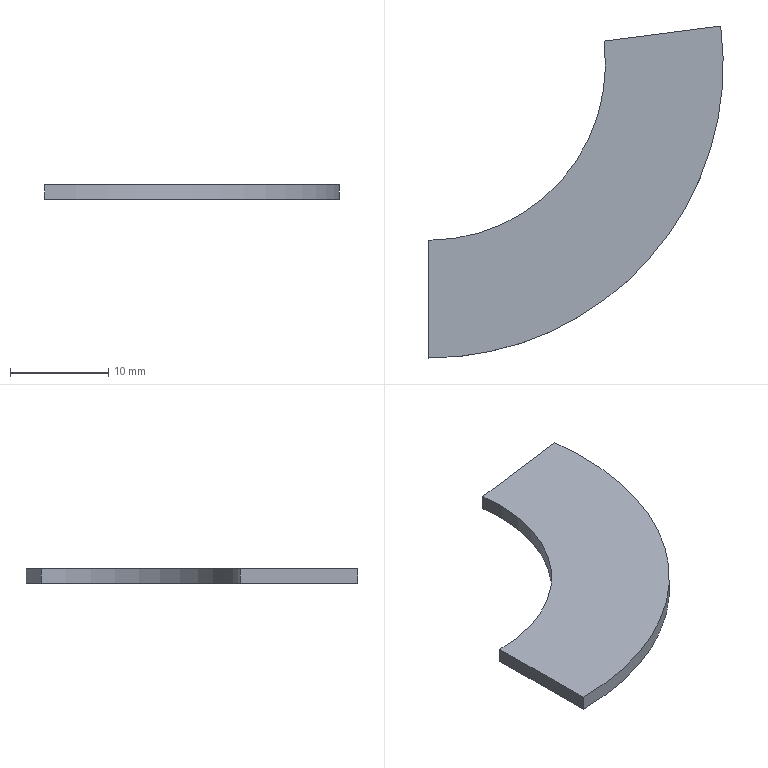Part | STEP file | FHD-021-012-F side door A-E | 1 solid | 6 faces | box 30 x 33.839 x 1.5 mm | volume 734.02 mm3 | plane 4 | cylinder 2 | commonest cylinder face diameters 36 x1 60 x1
STEP:
#1=CARTESIAN_POINT('',(0.,0.,0.));
#2=DIRECTION('',(0.,0.,1.));
#3=DIRECTION('',(1.,0.,0.));
#4=AXIS2_PLACEMENT_3D('',#1,#2,#3);
#5=CARTESIAN_POINT('',(1886.585,837.963,-1.5));
#6=VERTEX_POINT('',#5);
#7=CARTESIAN_POINT('',(1886.585,825.963,-1.5));
#8=VERTEX_POINT('',#7);
#9=CARTESIAN_POINT('',(1886.585,855.963,-1.5));
#10=DIRECTION('',(0.,-1.,0.));
#11=VECTOR('',#10,1.);
#12=LINE('',#9,#11);
#13=CARTESIAN_POINT('',(1886.585,855.963,-1.5));
#14=DIRECTION('',(0.,0.,1.));
#15=DIRECTION('',(1.,0.,0.));
#16=AXIS2_PLACEMENT_3D('',#13,#14,#15);
#17=PLANE('',#16);
#18=CARTESIAN_POINT('',(0.,0.));
#19=DIRECTION('',(0.,-1.));
#20=VECTOR('',#19,1.);
#21=LINE('',#18,#20);
#22=(GEOMETRIC_REPRESENTATION_CONTEXT(2)PARAMETRIC_REPRESENTATION_CONTEXT()REPRESENTATION_CONTEXT('',''));
#23=DEFINITIONAL_REPRESENTATION('',(#21),#22);
#24=PCURVE('',#17,#23);
#25=CARTESIAN_POINT('',(1886.585,837.963,-1.5));
#26=DIRECTION('',(-1.,0.,0.));
#27=DIRECTION('',(0.,0.,1.));
#28=AXIS2_PLACEMENT_3D('',#25,#26,#27);
#29=PLANE('',#28);
#30=CARTESIAN_POINT('',(0.,18.));
#31=DIRECTION('',(0.,-1.));
#32=VECTOR('',#31,1.);
#33=LINE('',#30,#32);
#34=(GEOMETRIC_REPRESENTATION_CONTEXT(2)PARAMETRIC_REPRESENTATION_CONTEXT()REPRESENTATION_CONTEXT('',''));
#35=DEFINITIONAL_REPRESENTATION('',(#33),#34);
#36=PCURVE('',#29,#35);
#37=SURFACE_CURVE('',#12,(#24,#36),.PCURVE_S1.);
#38=EDGE_CURVE('',#6,#8,#37,.T.);
#39=ORIENTED_EDGE('',*,*,#38,.F.);
#40=CARTESIAN_POINT('',(1904.437,858.266,-1.5));
#41=VERTEX_POINT('',#40);
#42=CARTESIAN_POINT('',(1886.585,855.963,-1.5));
#43=DIRECTION('',(0.,0.,-1.));
#44=DIRECTION('',(1.,0.,0.));
#45=AXIS2_PLACEMENT_3D('',#42,#43,#44);
#46=CIRCLE('',#45,18.);
#47=CARTESIAN_POINT('',(18.,0.));
#48=CARTESIAN_POINT('',(18.,-31.177));
#49=CARTESIAN_POINT('',(-9.,-15.588));
#50=CARTESIAN_POINT('',(-36.,0.));
#51=CARTESIAN_POINT('',(-9.,15.588));
#52=CARTESIAN_POINT('',(18.,31.177));
#53=CARTESIAN_POINT('',(18.,0.));
#54=(BOUNDED_CURVE()B_SPLINE_CURVE(2,(#47,#48,#49,#50,#51,#52,#53),.UNSPECIFIED.,.T.,.F.)B_SPLINE_CURVE_WITH_KNOTS((1,2,2,2,2,1),(-2.094,0.,2.094,4.189,6.283,8.378),.UNSPECIFIED.)CURVE()GEOMETRIC_REPRESENTATION_ITEM()RATIONAL_B_SPLINE_CURVE((1.,0.5,1.,0.5,1.,0.5,1.))REPRESENTATION_ITEM(''));
#55=(GEOMETRIC_REPRESENTATION_CONTEXT(2)PARAMETRIC_REPRESENTATION_CONTEXT()REPRESENTATION_CONTEXT('',''));
#56=DEFINITIONAL_REPRESENTATION('',(#54),#55);
#57=PCURVE('',#17,#56);
#58=CARTESIAN_POINT('',(1886.585,855.963,-1.5));
#59=DIRECTION('',(0.,0.,1.));
#60=DIRECTION('',(1.,0.,0.));
#61=AXIS2_PLACEMENT_3D('',#58,#59,#60);
#62=CYLINDRICAL_SURFACE('',#61,18.);
#63=CARTESIAN_POINT('',(12.566,0.));
#64=DIRECTION('',(-1.,0.));
#65=VECTOR('',#64,1.);
#66=LINE('',#63,#65);
#67=(GEOMETRIC_REPRESENTATION_CONTEXT(2)PARAMETRIC_REPRESENTATION_CONTEXT()REPRESENTATION_CONTEXT('',''));
#68=DEFINITIONAL_REPRESENTATION('',(#66),#67);
#69=PCURVE('',#62,#68);
#70=SURFACE_CURVE('',#46,(#57,#69),.PCURVE_S1.);
#71=EDGE_CURVE('',#41,#6,#70,.T.);
#72=ORIENTED_EDGE('',*,*,#71,.F.);
#73=CARTESIAN_POINT('',(1916.338,859.802,-1.5));
#74=VERTEX_POINT('',#73);
#75=CARTESIAN_POINT('',(1916.338,859.802,-1.5));
#76=DIRECTION('',(-0.9918,-0.128,0.));
#77=VECTOR('',#76,1.);
#78=LINE('',#75,#77);
#79=CARTESIAN_POINT('',(29.753,3.839));
#80=DIRECTION('',(-0.9918,-0.128));
#81=VECTOR('',#80,1.);
#82=LINE('',#79,#81);
#83=(GEOMETRIC_REPRESENTATION_CONTEXT(2)PARAMETRIC_REPRESENTATION_CONTEXT()REPRESENTATION_CONTEXT('',''));
#84=DEFINITIONAL_REPRESENTATION('',(#82),#83);
#85=PCURVE('',#17,#84);
#86=CARTESIAN_POINT('',(1916.338,859.802,-1.5));
#87=DIRECTION('',(-0.128,0.9918,0.));
#88=DIRECTION('',(-0.9918,-0.128,0.));
#89=AXIS2_PLACEMENT_3D('',#86,#87,#88);
#90=PLANE('',#89);
#91=CARTESIAN_POINT('',(0.,0.));
#92=DIRECTION('',(1.,0.));
#93=VECTOR('',#92,1.);
#94=LINE('',#91,#93);
#95=(GEOMETRIC_REPRESENTATION_CONTEXT(2)PARAMETRIC_REPRESENTATION_CONTEXT()REPRESENTATION_CONTEXT('',''));
#96=DEFINITIONAL_REPRESENTATION('',(#94),#95);
#97=PCURVE('',#90,#96);
#98=SURFACE_CURVE('',#78,(#85,#97),.PCURVE_S1.);
#99=EDGE_CURVE('',#74,#41,#98,.T.);
#100=ORIENTED_EDGE('',*,*,#99,.F.);
#101=CARTESIAN_POINT('',(1886.585,855.963,-1.5));
#102=DIRECTION('',(0.,0.,1.));
#103=DIRECTION('',(1.,0.,0.));
#104=AXIS2_PLACEMENT_3D('',#101,#102,#103);
#105=CIRCLE('',#104,30.);
#106=CARTESIAN_POINT('',(0.,0.));
#107=DIRECTION('',(1.,0.));
#108=AXIS2_PLACEMENT_2D('',#106,#107);
#109=CIRCLE('',#108,30.);
#110=(GEOMETRIC_REPRESENTATION_CONTEXT(2)PARAMETRIC_REPRESENTATION_CONTEXT()REPRESENTATION_CONTEXT('',''));
#111=DEFINITIONAL_REPRESENTATION('',(#109),#110);
#112=PCURVE('',#17,#111);
#113=CARTESIAN_POINT('',(1886.585,855.963,-1.5));
#114=DIRECTION('',(0.,0.,1.));
#115=DIRECTION('',(1.,0.,0.));
#116=AXIS2_PLACEMENT_3D('',#113,#114,#115);
#117=CYLINDRICAL_SURFACE('',#116,30.);
#118=CARTESIAN_POINT('',(0.,0.));
#119=DIRECTION('',(1.,0.));
#120=VECTOR('',#119,1.);
#121=LINE('',#118,#120);
#122=(GEOMETRIC_REPRESENTATION_CONTEXT(2)PARAMETRIC_REPRESENTATION_CONTEXT()REPRESENTATION_CONTEXT('',''));
#123=DEFINITIONAL_REPRESENTATION('',(#121),#122);
#124=PCURVE('',#117,#123);
#125=SURFACE_CURVE('',#105,(#112,#124),.PCURVE_S1.);
#126=EDGE_CURVE('',#8,#74,#125,.T.);
#127=ORIENTED_EDGE('',*,*,#126,.F.);
#128=EDGE_LOOP('',(#39,#72,#100,#127));
#129=FACE_BOUND('',#128,.T.);
#130=ADVANCED_FACE('',(#129),#17,.F.);
#131=CARTESIAN_POINT('',(1916.338,859.802,0.));
#132=VERTEX_POINT('',#131);
#133=CARTESIAN_POINT('',(1886.585,825.963,0.));
#134=VERTEX_POINT('',#133);
#135=CARTESIAN_POINT('',(1886.585,855.963,0.));
#136=DIRECTION('',(0.,0.,-1.));
#137=DIRECTION('',(1.,0.,0.));
#138=AXIS2_PLACEMENT_3D('',#135,#136,#137);
#139=CIRCLE('',#138,30.);
#140=CARTESIAN_POINT('',(12.566,1.5));
#141=DIRECTION('',(-1.,0.));
#142=VECTOR('',#141,1.);
#143=LINE('',#140,#142);
#144=(GEOMETRIC_REPRESENTATION_CONTEXT(2)PARAMETRIC_REPRESENTATION_CONTEXT()REPRESENTATION_CONTEXT('',''));
#145=DEFINITIONAL_REPRESENTATION('',(#143),#144);
#146=PCURVE('',#117,#145);
#147=CARTESIAN_POINT('',(1886.585,855.963,0.));
#148=DIRECTION('',(0.,0.,1.));
#149=DIRECTION('',(1.,0.,0.));
#150=AXIS2_PLACEMENT_3D('',#147,#148,#149);
#151=PLANE('',#150);
#152=CARTESIAN_POINT('',(30.,0.));
#153=CARTESIAN_POINT('',(30.,-51.962));
#154=CARTESIAN_POINT('',(-15.,-25.981));
#155=CARTESIAN_POINT('',(-60.,0.));
#156=CARTESIAN_POINT('',(-15.,25.981));
#157=CARTESIAN_POINT('',(30.,51.962));
#158=CARTESIAN_POINT('',(30.,0.));
#159=(BOUNDED_CURVE()B_SPLINE_CURVE(2,(#152,#153,#154,#155,#156,#157,#158),.UNSPECIFIED.,.T.,.F.)B_SPLINE_CURVE_WITH_KNOTS((1,2,2,2,2,1),(-2.094,0.,2.094,4.189,6.283,8.378),.UNSPECIFIED.)CURVE()GEOMETRIC_REPRESENTATION_ITEM()RATIONAL_B_SPLINE_CURVE((1.,0.5,1.,0.5,1.,0.5,1.))REPRESENTATION_ITEM(''));
#160=(GEOMETRIC_REPRESENTATION_CONTEXT(2)PARAMETRIC_REPRESENTATION_CONTEXT()REPRESENTATION_CONTEXT('',''));
#161=DEFINITIONAL_REPRESENTATION('',(#159),#160);
#162=PCURVE('',#151,#161);
#163=SURFACE_CURVE('',#139,(#146,#162),.PCURVE_S1.);
#164=EDGE_CURVE('',#132,#134,#163,.T.);
#165=ORIENTED_EDGE('',*,*,#164,.T.);
#166=CARTESIAN_POINT('',(1886.585,825.963,-1.5));
#167=DIRECTION('',(0.,0.,-1.));
#168=VECTOR('',#167,1.);
#169=LINE('',#166,#168);
#170=CARTESIAN_POINT('',(4.712,0.));
#171=DIRECTION('',(0.,-1.));
#172=VECTOR('',#171,1.);
#173=LINE('',#170,#172);
#174=(GEOMETRIC_REPRESENTATION_CONTEXT(2)PARAMETRIC_REPRESENTATION_CONTEXT()REPRESENTATION_CONTEXT('',''));
#175=DEFINITIONAL_REPRESENTATION('',(#173),#174);
#176=PCURVE('',#117,#175);
#177=CARTESIAN_POINT('',(0.,-12.));
#178=DIRECTION('',(-1.,0.));
#179=VECTOR('',#178,1.);
#180=LINE('',#177,#179);
#181=(GEOMETRIC_REPRESENTATION_CONTEXT(2)PARAMETRIC_REPRESENTATION_CONTEXT()REPRESENTATION_CONTEXT('',''));
#182=DEFINITIONAL_REPRESENTATION('',(#180),#181);
#183=PCURVE('',#29,#182);
#184=SURFACE_CURVE('',#169,(#176,#183),.PCURVE_S1.);
#185=EDGE_CURVE('',#134,#8,#184,.T.);
#186=ORIENTED_EDGE('',*,*,#185,.T.);
#187=ORIENTED_EDGE('',*,*,#126,.T.);
#188=CARTESIAN_POINT('',(1916.338,859.802,-1.5));
#189=DIRECTION('',(0.,0.,-1.));
#190=VECTOR('',#189,1.);
#191=LINE('',#188,#190);
#192=CARTESIAN_POINT('',(6.412,0.));
#193=DIRECTION('',(0.,-1.));
#194=VECTOR('',#193,1.);
#195=LINE('',#192,#194);
#196=(GEOMETRIC_REPRESENTATION_CONTEXT(2)PARAMETRIC_REPRESENTATION_CONTEXT()REPRESENTATION_CONTEXT('',''));
#197=DEFINITIONAL_REPRESENTATION('',(#195),#196);
#198=PCURVE('',#117,#197);
#199=CARTESIAN_POINT('',(0.,0.));
#200=DIRECTION('',(0.,-1.));
#201=VECTOR('',#200,1.);
#202=LINE('',#199,#201);
#203=(GEOMETRIC_REPRESENTATION_CONTEXT(2)PARAMETRIC_REPRESENTATION_CONTEXT()REPRESENTATION_CONTEXT('',''));
#204=DEFINITIONAL_REPRESENTATION('',(#202),#203);
#205=PCURVE('',#90,#204);
#206=SURFACE_CURVE('',#191,(#198,#205),.PCURVE_S1.);
#207=EDGE_CURVE('',#132,#74,#206,.T.);
#208=ORIENTED_EDGE('',*,*,#207,.F.);
#209=EDGE_LOOP('',(#165,#186,#187,#208));
#210=FACE_BOUND('',#209,.T.);
#211=ADVANCED_FACE('',(#210),#117,.T.);
#212=ORIENTED_EDGE('',*,*,#38,.T.);
#213=ORIENTED_EDGE('',*,*,#185,.F.);
#214=CARTESIAN_POINT('',(1886.585,837.963,0.));
#215=VERTEX_POINT('',#214);
#216=CARTESIAN_POINT('',(1886.585,837.963,0.));
#217=DIRECTION('',(0.,1.,0.));
#218=VECTOR('',#217,1.);
#219=LINE('',#216,#218);
#220=CARTESIAN_POINT('',(1.5,0.));
#221=DIRECTION('',(0.,1.));
#222=VECTOR('',#221,1.);
#223=LINE('',#220,#222);
#224=(GEOMETRIC_REPRESENTATION_CONTEXT(2)PARAMETRIC_REPRESENTATION_CONTEXT()REPRESENTATION_CONTEXT('',''));
#225=DEFINITIONAL_REPRESENTATION('',(#223),#224);
#226=PCURVE('',#29,#225);
#227=CARTESIAN_POINT('',(0.,-18.));
#228=DIRECTION('',(0.,1.));
#229=VECTOR('',#228,1.);
#230=LINE('',#227,#229);
#231=(GEOMETRIC_REPRESENTATION_CONTEXT(2)PARAMETRIC_REPRESENTATION_CONTEXT()REPRESENTATION_CONTEXT('',''));
#232=DEFINITIONAL_REPRESENTATION('',(#230),#231);
#233=PCURVE('',#151,#232);
#234=SURFACE_CURVE('',#219,(#226,#233),.PCURVE_S1.);
#235=EDGE_CURVE('',#134,#215,#234,.T.);
#236=ORIENTED_EDGE('',*,*,#235,.T.);
#237=CARTESIAN_POINT('',(1886.585,837.963,-1.5));
#238=DIRECTION('',(0.,0.,-1.));
#239=VECTOR('',#238,1.);
#240=LINE('',#237,#239);
#241=CARTESIAN_POINT('',(0.,0.));
#242=DIRECTION('',(-1.,0.));
#243=VECTOR('',#242,1.);
#244=LINE('',#241,#243);
#245=(GEOMETRIC_REPRESENTATION_CONTEXT(2)PARAMETRIC_REPRESENTATION_CONTEXT()REPRESENTATION_CONTEXT('',''));
#246=DEFINITIONAL_REPRESENTATION('',(#244),#245);
#247=PCURVE('',#29,#246);
#248=CARTESIAN_POINT('',(4.712,0.));
#249=DIRECTION('',(0.,-1.));
#250=VECTOR('',#249,1.);
#251=LINE('',#248,#250);
#252=(GEOMETRIC_REPRESENTATION_CONTEXT(2)PARAMETRIC_REPRESENTATION_CONTEXT()REPRESENTATION_CONTEXT('',''));
#253=DEFINITIONAL_REPRESENTATION('',(#251),#252);
#254=PCURVE('',#62,#253);
#255=SURFACE_CURVE('',#240,(#247,#254),.PCURVE_S1.);
#256=EDGE_CURVE('',#215,#6,#255,.T.);
#257=ORIENTED_EDGE('',*,*,#256,.T.);
#258=EDGE_LOOP('',(#212,#213,#236,#257));
#259=FACE_BOUND('',#258,.T.);
#260=ADVANCED_FACE('',(#259),#29,.T.);
#261=CARTESIAN_POINT('',(1904.437,858.266,0.));
#262=VERTEX_POINT('',#261);
#263=CARTESIAN_POINT('',(1904.437,858.266,-1.5));
#264=DIRECTION('',(0.,0.,1.));
#265=VECTOR('',#264,1.);
#266=LINE('',#263,#265);
#267=CARTESIAN_POINT('',(6.412,0.));
#268=DIRECTION('',(0.,1.));
#269=VECTOR('',#268,1.);
#270=LINE('',#267,#269);
#271=(GEOMETRIC_REPRESENTATION_CONTEXT(2)PARAMETRIC_REPRESENTATION_CONTEXT()REPRESENTATION_CONTEXT('',''));
#272=DEFINITIONAL_REPRESENTATION('',(#270),#271);
#273=PCURVE('',#62,#272);
#274=CARTESIAN_POINT('',(12.,0.));
#275=DIRECTION('',(0.,1.));
#276=VECTOR('',#275,1.);
#277=LINE('',#274,#276);
#278=(GEOMETRIC_REPRESENTATION_CONTEXT(2)PARAMETRIC_REPRESENTATION_CONTEXT()REPRESENTATION_CONTEXT('',''));
#279=DEFINITIONAL_REPRESENTATION('',(#277),#278);
#280=PCURVE('',#90,#279);
#281=SURFACE_CURVE('',#266,(#273,#280),.PCURVE_S1.);
#282=EDGE_CURVE('',#41,#262,#281,.T.);
#283=ORIENTED_EDGE('',*,*,#282,.T.);
#284=CARTESIAN_POINT('',(1886.585,855.963,0.));
#285=DIRECTION('',(0.,0.,-1.));
#286=DIRECTION('',(1.,0.,0.));
#287=AXIS2_PLACEMENT_3D('',#284,#285,#286);
#288=CIRCLE('',#287,18.);
#289=CARTESIAN_POINT('',(12.566,1.5));
#290=DIRECTION('',(-1.,0.));
#291=VECTOR('',#290,1.);
#292=LINE('',#289,#291);
#293=(GEOMETRIC_REPRESENTATION_CONTEXT(2)PARAMETRIC_REPRESENTATION_CONTEXT()REPRESENTATION_CONTEXT('',''));
#294=DEFINITIONAL_REPRESENTATION('',(#292),#293);
#295=PCURVE('',#62,#294);
#296=CARTESIAN_POINT('',(18.,0.));
#297=CARTESIAN_POINT('',(18.,-31.177));
#298=CARTESIAN_POINT('',(-9.,-15.588));
#299=CARTESIAN_POINT('',(-36.,0.));
#300=CARTESIAN_POINT('',(-9.,15.588));
#301=CARTESIAN_POINT('',(18.,31.177));
#302=CARTESIAN_POINT('',(18.,0.));
#303=(BOUNDED_CURVE()B_SPLINE_CURVE(2,(#296,#297,#298,#299,#300,#301,#302),.UNSPECIFIED.,.T.,.F.)B_SPLINE_CURVE_WITH_KNOTS((1,2,2,2,2,1),(-2.094,0.,2.094,4.189,6.283,8.378),.UNSPECIFIED.)CURVE()GEOMETRIC_REPRESENTATION_ITEM()RATIONAL_B_SPLINE_CURVE((1.,0.5,1.,0.5,1.,0.5,1.))REPRESENTATION_ITEM(''));
#304=(GEOMETRIC_REPRESENTATION_CONTEXT(2)PARAMETRIC_REPRESENTATION_CONTEXT()REPRESENTATION_CONTEXT('',''));
#305=DEFINITIONAL_REPRESENTATION('',(#303),#304);
#306=PCURVE('',#151,#305);
#307=SURFACE_CURVE('',#288,(#295,#306),.PCURVE_S1.);
#308=EDGE_CURVE('',#262,#215,#307,.T.);
#309=ORIENTED_EDGE('',*,*,#308,.T.);
#310=ORIENTED_EDGE('',*,*,#256,.T.);
#311=ORIENTED_EDGE('',*,*,#71,.F.);
#312=EDGE_LOOP('',(#283,#309,#310,#311));
#313=FACE_BOUND('',#312,.F.);
#314=ADVANCED_FACE('',(#313),#62,.F.);
#315=ORIENTED_EDGE('',*,*,#99,.T.);
#316=ORIENTED_EDGE('',*,*,#282,.T.);
#317=CARTESIAN_POINT('',(1916.338,859.802,0.));
#318=DIRECTION('',(0.9918,0.128,0.));
#319=VECTOR('',#318,1.);
#320=LINE('',#317,#319);
#321=CARTESIAN_POINT('',(0.,1.5));
#322=DIRECTION('',(-1.,0.));
#323=VECTOR('',#322,1.);
#324=LINE('',#321,#323);
#325=(GEOMETRIC_REPRESENTATION_CONTEXT(2)PARAMETRIC_REPRESENTATION_CONTEXT()REPRESENTATION_CONTEXT('',''));
#326=DEFINITIONAL_REPRESENTATION('',(#324),#325);
#327=PCURVE('',#90,#326);
#328=CARTESIAN_POINT('',(29.753,3.839));
#329=DIRECTION('',(0.9918,0.128));
#330=VECTOR('',#329,1.);
#331=LINE('',#328,#330);
#332=(GEOMETRIC_REPRESENTATION_CONTEXT(2)PARAMETRIC_REPRESENTATION_CONTEXT()REPRESENTATION_CONTEXT('',''));
#333=DEFINITIONAL_REPRESENTATION('',(#331),#332);
#334=PCURVE('',#151,#333);
#335=SURFACE_CURVE('',#320,(#327,#334),.PCURVE_S1.);
#336=EDGE_CURVE('',#262,#132,#335,.T.);
#337=ORIENTED_EDGE('',*,*,#336,.T.);
#338=ORIENTED_EDGE('',*,*,#207,.T.);
#339=EDGE_LOOP('',(#315,#316,#337,#338));
#340=FACE_BOUND('',#339,.T.);
#341=ADVANCED_FACE('',(#340),#90,.T.);
#342=ORIENTED_EDGE('',*,*,#308,.T.);
#343=ORIENTED_EDGE('',*,*,#235,.F.);
#344=ORIENTED_EDGE('',*,*,#164,.F.);
#345=ORIENTED_EDGE('',*,*,#336,.F.);
#346=EDGE_LOOP('',(#342,#343,#344,#345));
#347=FACE_BOUND('',#346,.T.);
#348=ADVANCED_FACE('',(#347),#151,.T.);
#349=CLOSED_SHELL('',(#130,#211,#260,#314,#341,#348));
#350=MANIFOLD_SOLID_BREP('',#349);
#351=(LENGTH_UNIT()NAMED_UNIT(*)SI_UNIT(.MILLI.,.METRE.));
#352=UNCERTAINTY_MEASURE_WITH_UNIT(LENGTH_MEASURE(0.0000001),#351,'','');
#353=(NAMED_UNIT(*)PLANE_ANGLE_UNIT()SI_UNIT($,.RADIAN.));
#354=(NAMED_UNIT(*)SI_UNIT($,.STERADIAN.)SOLID_ANGLE_UNIT());
#355=(GEOMETRIC_REPRESENTATION_CONTEXT(3)GLOBAL_UNCERTAINTY_ASSIGNED_CONTEXT((#352))GLOBAL_UNIT_ASSIGNED_CONTEXT((#351,#353,#354))REPRESENTATION_CONTEXT('',''));
#356=ADVANCED_BREP_SHAPE_REPRESENTATION('',(#4,#350),#355);